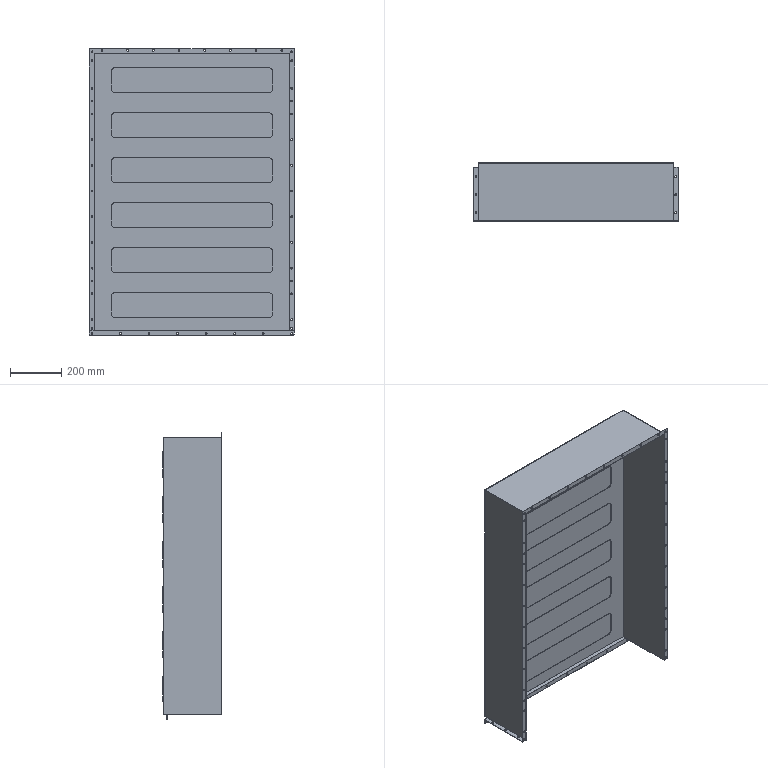Part | NX | features BREP 1 | 1 solid | 287 faces | box 798.2 x 228.75 x 1116 mm | volume 1898468 mm3 | cylinder 180 | plane 83 | torus 24 | commonest cylinder face diameters 7 x104 2 x24 27 x24 30 x24 10 x4